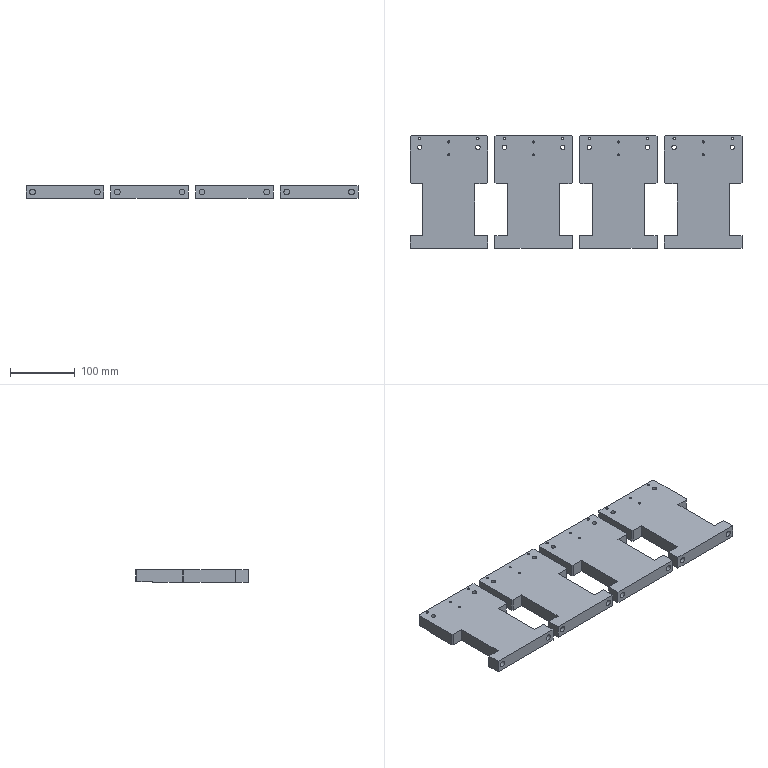CAM job | NX | 3-axis milling, drilling | part box 513 x 174.5 x 20 mm | stock box 518 x 179.5 x 20 mm
Tools:
number,name,description,diameter,corner_radius,flute_length,length,flutes
9,D10,平底铣刀-粗,10.0,0.0,35.0,75.0,2
11,D4-J,平底铣刀-精,4.0,0.0,50.0,75.0,2
7,D6-J,平底铣刀-精,6.0,0.0,25.0,75.0,2
10,D10-J,平底铣刀-精,10.0,0.0,35.0,75.0,2
1,D80R0.8FACEMILL-J,圆鼻刀-精,80.0,0.8,50.0,75.0,2
2,D6CHAMFERMILL,倒角刀,6.0,0.0,3.0,25.0,2
21,M4X0.7,丝锥,3.3,0.0,35.0,50.0,2
13,ZT3.4,钻头,3.4,0.0,35.0,50.0,2
18,ZT3.6,钻头,3.6,0.0,35.0,50.0,2
17,ZT7,钻头,7.0,0.0,35.0,50.0,2
Operations:
program,operation,operation_type,tool,method,geometry_group,spindle_rpm,surface_speed,feed_per_tooth,feed_cut,feed_plunge,cut_length_mm,path_length_mm,cut_time_min,machine_time_min
C,FLOORWALLFINISH-FLOORMID_COPY,VolumeBased25DMillingOperation,D10-J,FINISHSTEPDEPTHOFF,W-C,8000.0,251.32,0.0625,1000.0,100.0,758.603,779.403,0.7586,0.7607
C,FLOORWALLFINISH-SIDEMID-SELFLOOR_COPY,VolumeBased25DMillingOperation,D10-J,SIDEFINISH-DEPTHK-STEPG,W-C,8000.0,251.32,0.0625,1000.0,100.0,138.681,160.681,0.1387,0.1409
A,FLOORWALLFACEFINISH_COPY,VolumeBased25DMillingOperation,D80R0.8FACEMILL-J,SIDEFINISH-DEPTHK-STEPG,W-A,4000.0,1005.28,0.125,1000.0,100.0,1912.397,1968.397,1.912,1.918
A,FLOORWALLROUGH_1,VolumeBased25DMillingOperation,D10,METHOD,W-A,8000.0,251.327,0.2812,4500.0,100.0,6745.185,7804.452,1.499,1.605
A,PROFILEROUGH_2,VolumeBased25DMillingOperation,D10,METHOD,W-A,8000.0,251.327,0.3125,5000.0,80.0,112772.789,113476.289,22.555,22.625
A,SPOTDRILL-DEPTH0.8,Operation,D6CHAMFERMILL,NONE,W-A,8000.0,201.062,0.0156,500.0,90.0,14.4,581.859,0.0288,0.0855
A,4_THROUGHHOLE-6-8,Operation,ZT7,NONE,W-A,2000.0,43.982,0.0375,150.0,90.0,28.0,609.059,0.1867,0.2448
A,FLOORFINISH_1,VolumeBased25DMillingOperation,D6-J,METHOD,W-A,6000.0,113.0,0.2083,1200.0,100.0,3945.78,4590.174,3.288,3.353
A,FLOORSIDEFINISH_3,VolumeBased25DMillingOperation,D6-J,METHOD,W-A,6000.0,113.0,0.2083,1200.0,100.0,518.966,1542.126,0.4325,0.5348
A,PROFILED4CORNER,ZLevelMilling,D4-J,METHOD,W-A,8000.0,100.531,0.1562,2500.0,80.0,11780.483,14121.524,4.714,4.948
A,CHAMFER_2,SurfaceContour,D6CHAMFERMILL,METHOD,W-A,6000.0,113.0,0.125,1200.0,100.0,3230.394,4999.741,2.692,2.869
A,DRILLCHAMFER_1,Operation,D6CHAMFERMILL,METHOD,W-A,8000.0,150.796,0.0625,1000.0,0.0,41.6,641.415,0.0416,0.1016
A,DRILLCHAMFER_2,Operation,D6CHAMFERMILL,METHOD,W-A,8000.0,150.796,0.0625,1000.0,0.0,40.8,649.129,0.0408,0.1016
A,MILLCHAMFER_1,PlanarMilling,D6CHAMFERMILL,METHOD,W-A,8000.0,150.796,0.075,1200.0,100.0,171.925,1173.664,0.1433,0.2434
A,PROFILESEMIFINISH_2,VolumeBased25DMillingOperation,D6-J,METHOD,W-A,6000.0,113.0,0.0833,1000.0,100.0,5463.433,6580.066,5.463,5.575
A,PROFILEFINISH_2,VolumeBased25DMillingOperation,D6-J,METHOD,W-A,6000.0,113.0,0.0833,1000.0,100.0,2730.916,3525.831,2.731,2.81
B,SPOTDRILL-DEPTH0.8_2,Operation,D6CHAMFERMILL,NONE,W-B,8000.0,150.796,0.0312,500.0,90.0,10.8,225.572,0.0216,0.0431
B,THROUGHHOLE-M4TAPDRILL,Operation,ZT3.4,NONE,W-B,3000.0,31.102,0.05,300.0,90.0,52.0,185.025,0.1733,0.1866
B,THROUGHHOLE-3-4,Operation,ZT3.6,NONE,W-B,3000.0,33.929,0.02,120.0,90.0,45.163,241.332,0.3764,0.396
B,THROUGHHOLE-6-8,Operation,ZT7,NONE,W-B,2500.0,54.978,0.03,150.0,90.0,47.206,245.418,0.3147,0.3345
B,DRILLCHAMFER_3,Operation,D6CHAMFERMILL,METHOD,W-B,8000.0,150.796,0.0312,500.0,0.0,10.4,104.024,0.0208,0.0302
B,DRILLCHAMFER_4,Operation,D6CHAMFERMILL,METHOD,W-B,8000.0,150.796,0.0312,500.0,0.0,10.2,173.45,0.0204,0.0367
B,MILLCHAMFER_2,PlanarMilling,D6CHAMFERMILL,METHOD,W-B,8000.0,150.796,0.05,800.0,100.0,47.831,259.881,0.0598,0.081
B,PLANEDEBURR6X45L_COPY,SurfaceContour,D6CHAMFERMILL,CREEPCHAMFER-DEPTH0-STEPG,W-B,8000.0,150.796,0.0938,1500.0,100.0,750.527,1230.189,0.5004,0.5483
B,THROUGHHOLE-TAPM4,Operation,M4X0.7,METHOD,W-B,600.0,6.22,0.0006,0.7,90.0,46.5,174.025,66.429,66.441